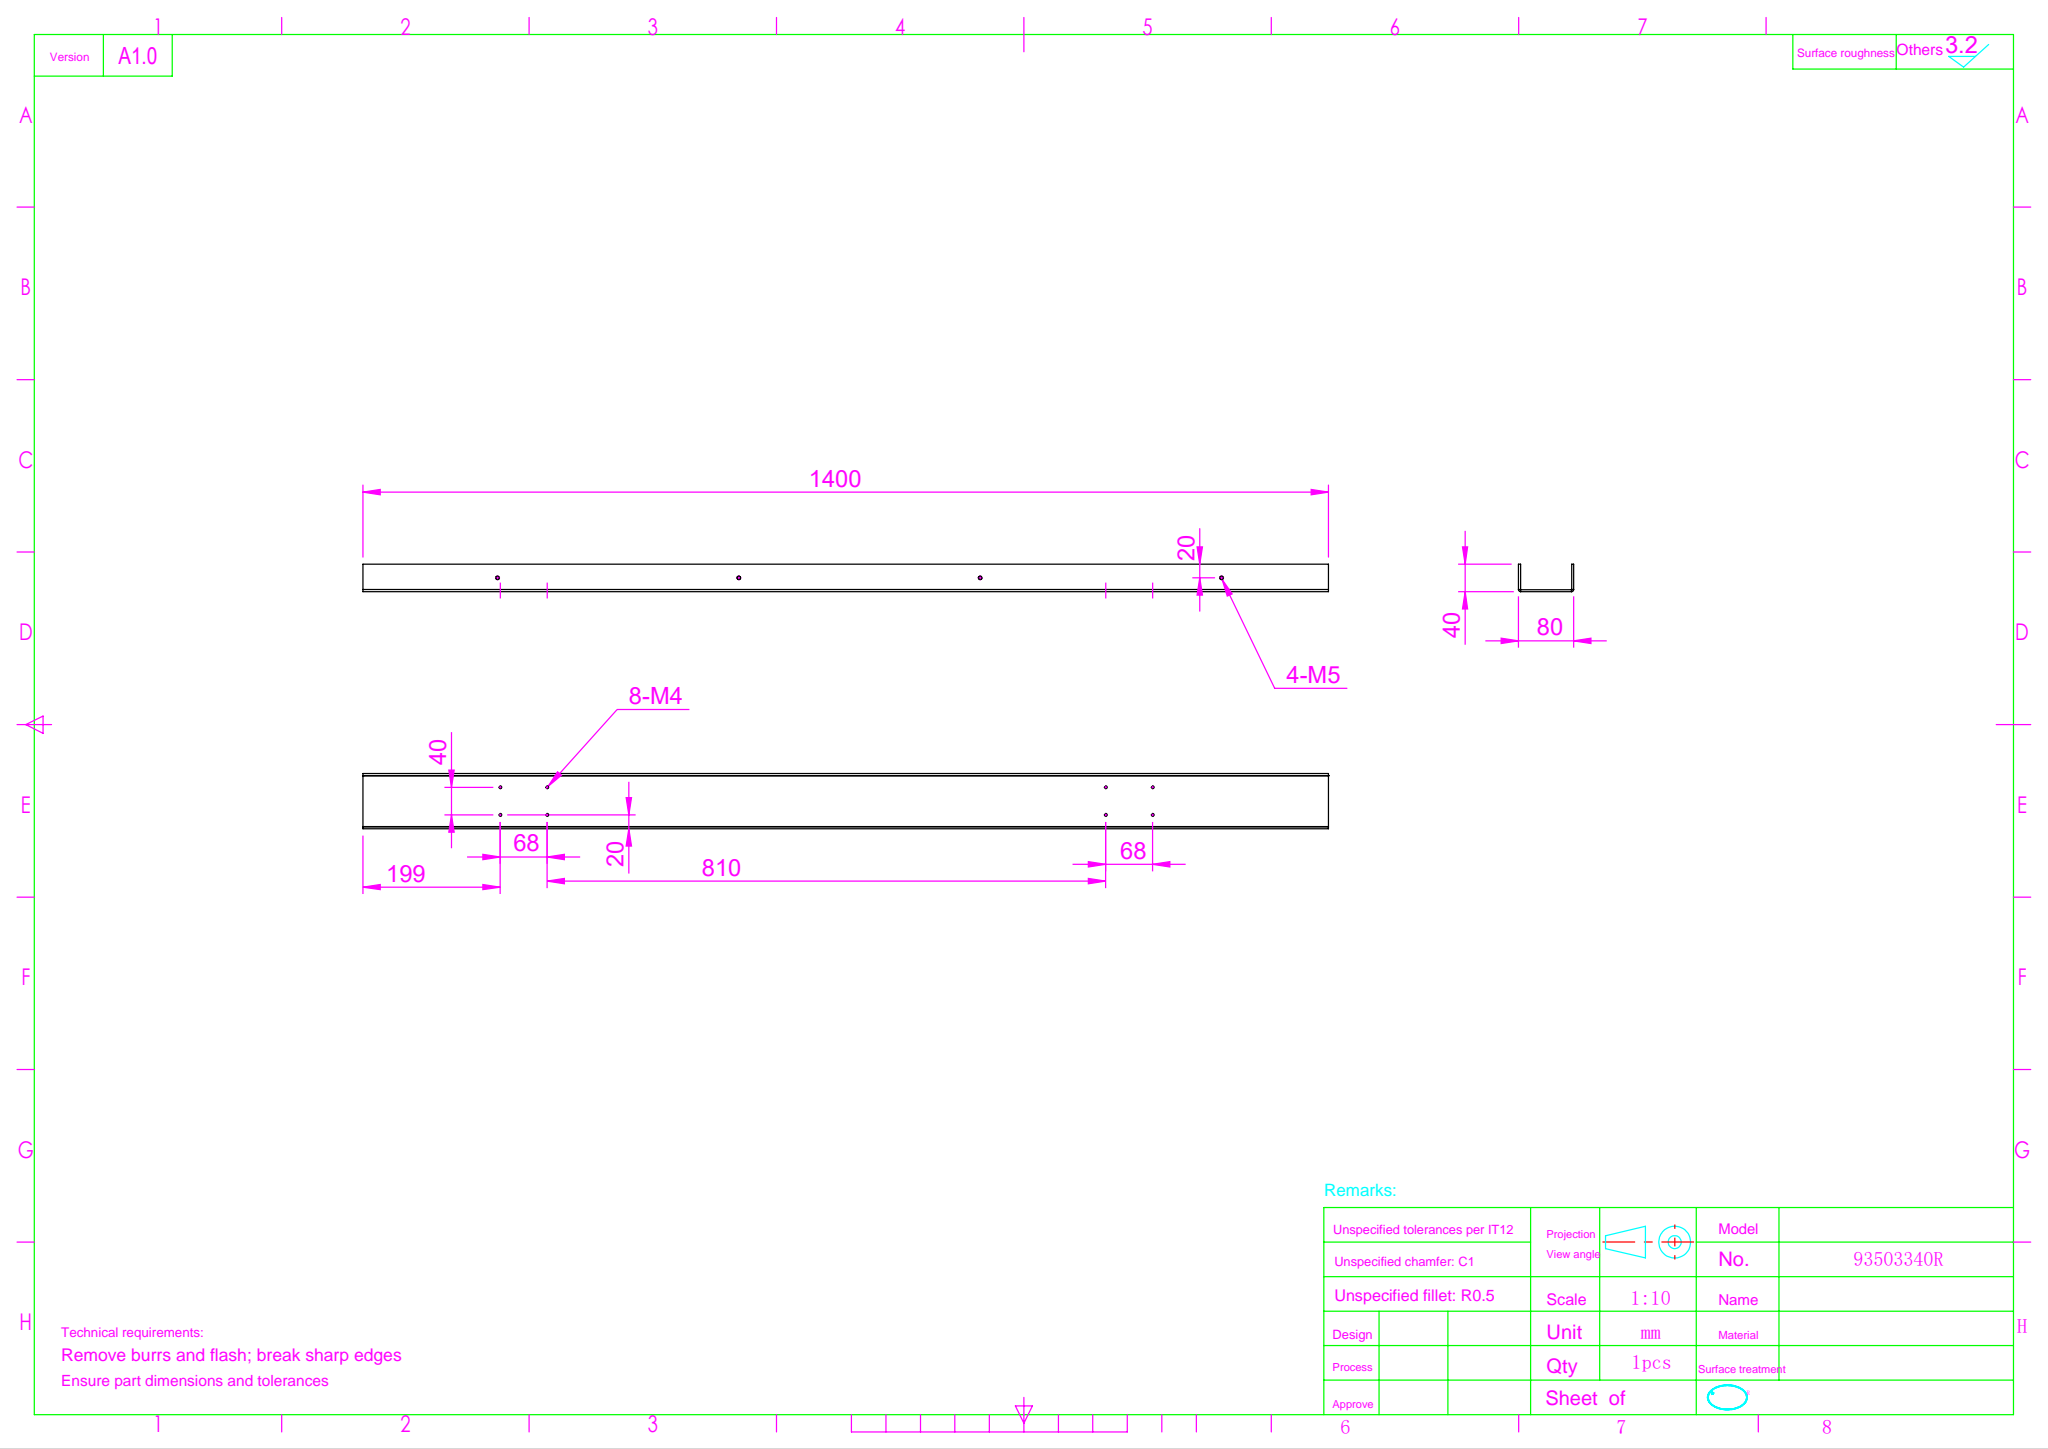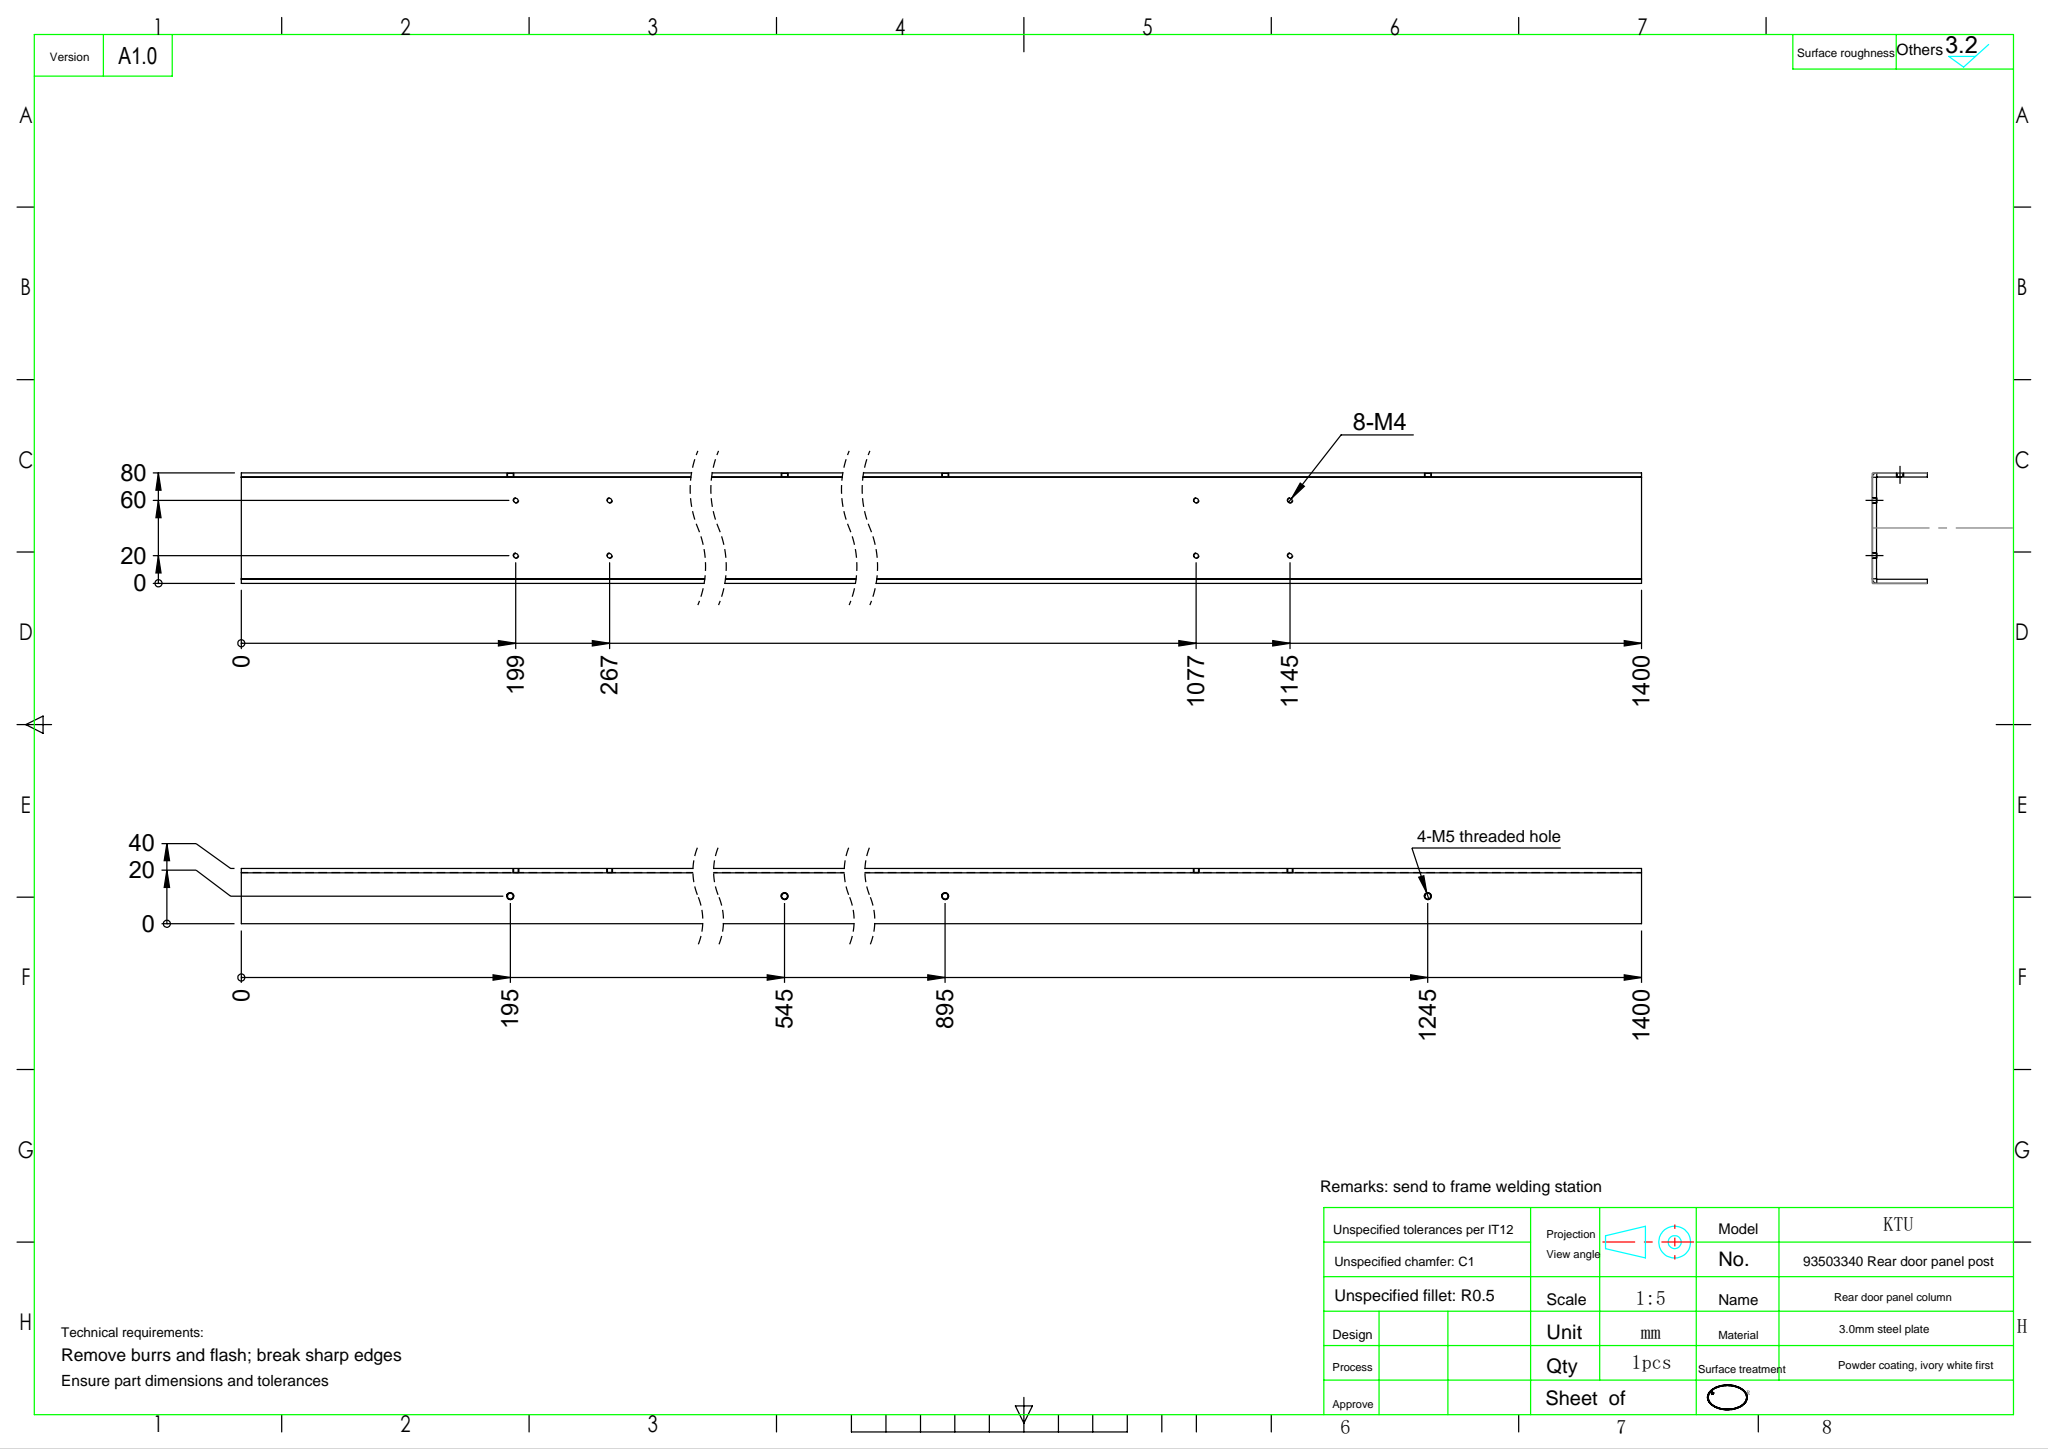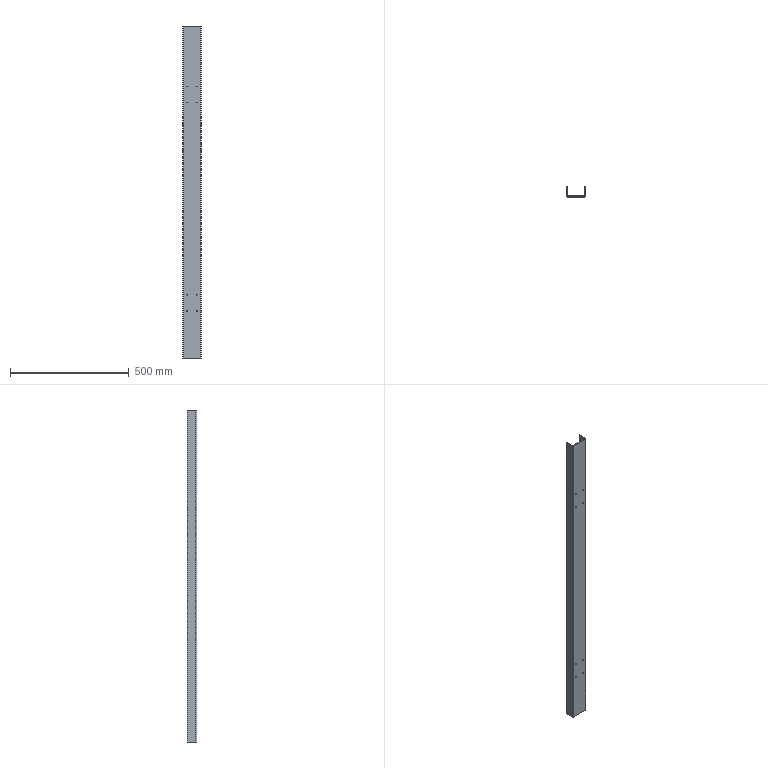Part | SolidWorks | features HoleWzd 2, 3DProfileFeature 1, Cut 1, DelFace 1, FlatPattern 1, SMBaseFlange 1, SheetMetal 1 | 1 solid | 54 faces | box 80 x 40 x 1400 mm | volume 640294 mm3 | cylinder 28 | plane 18 | cone 8 | commonest cylinder face diameters 3.3 x16 4.2 x8 0.4 x2 6.4 x2